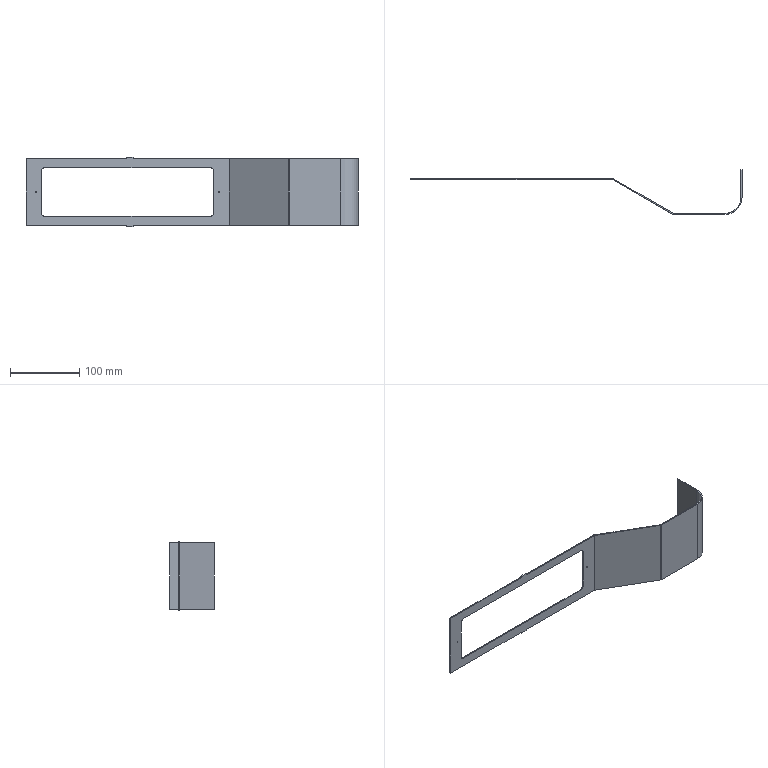Part | STEP file | FHD-021-001-L rack welded part L | 1 solid | 36 faces | box 480.9 x 65 x 100 mm | volume 53460 mm3 | plane 24 | cylinder 12 | commonest cylinder face diameters 10 x4 0.4 x2 2 x2 3.4 x2 47 x1 50 x1